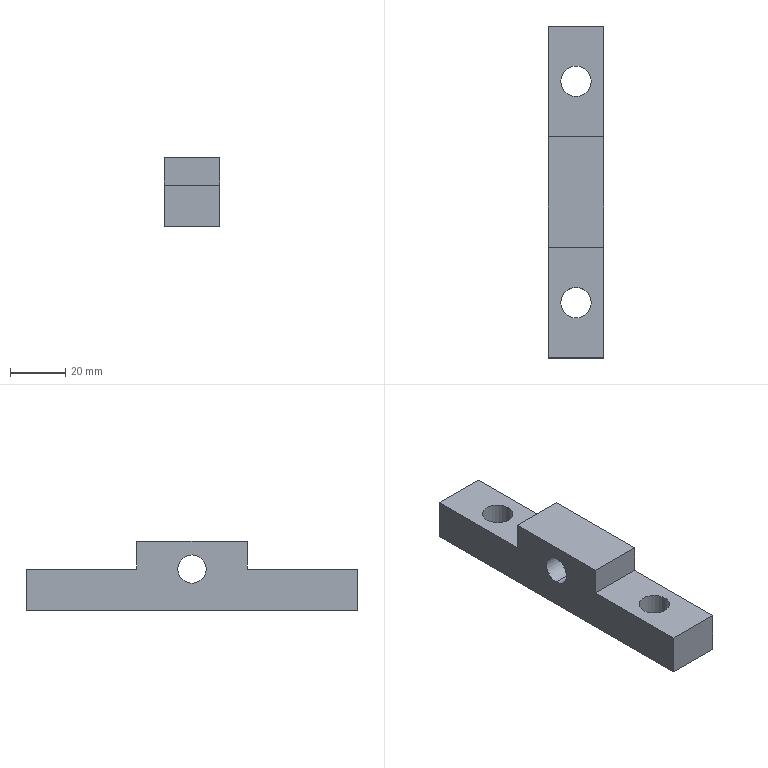Part | STEP file | Driven sprocket expansion seat | 1 solid | 16 faces | box 20 x 120 x 25 mm | volume 39515 mm3 | plane 10 | cylinder 6 | commonest cylinder face diameters 11 x4 10.2 x2
STEP:
#1=CARTESIAN_POINT('',(0.,0.,0.));
#2=DIRECTION('',(0.,0.,1.));
#3=DIRECTION('',(1.,0.,0.));
#4=AXIS2_PLACEMENT_3D('',#1,#2,#3);
#5=CARTESIAN_POINT('',(-10.,0.,9.9));
#6=VERTEX_POINT('',#5);
#7=CARTESIAN_POINT('',(10.,0.,9.9));
#8=VERTEX_POINT('',#7);
#9=CARTESIAN_POINT('',(10.,0.,9.9));
#10=DIRECTION('',(1.,0.,0.));
#11=VECTOR('',#10,1.);
#12=LINE('',#9,#11);
#13=CARTESIAN_POINT('',(10.,0.,15.));
#14=DIRECTION('',(1.,0.,0.));
#15=DIRECTION('',(0.,0.,-1.));
#16=AXIS2_PLACEMENT_3D('',#13,#14,#15);
#17=CYLINDRICAL_SURFACE('',#16,5.1);
#18=CARTESIAN_POINT('',(6.283,0.));
#19=DIRECTION('',(0.,1.));
#20=VECTOR('',#19,1.);
#21=LINE('',#18,#20);
#22=(GEOMETRIC_REPRESENTATION_CONTEXT(2)PARAMETRIC_REPRESENTATION_CONTEXT()REPRESENTATION_CONTEXT('',''));
#23=DEFINITIONAL_REPRESENTATION('',(#21),#22);
#24=PCURVE('',#17,#23);
#25=CARTESIAN_POINT('',(10.,0.,15.));
#26=DIRECTION('',(1.,0.,0.));
#27=DIRECTION('',(0.,0.,-1.));
#28=AXIS2_PLACEMENT_3D('',#25,#26,#27);
#29=CYLINDRICAL_SURFACE('',#28,5.1);
#30=CARTESIAN_POINT('',(0.,0.));
#31=DIRECTION('',(0.,1.));
#32=VECTOR('',#31,1.);
#33=LINE('',#30,#32);
#34=(GEOMETRIC_REPRESENTATION_CONTEXT(2)PARAMETRIC_REPRESENTATION_CONTEXT()REPRESENTATION_CONTEXT('',''));
#35=DEFINITIONAL_REPRESENTATION('',(#33),#34);
#36=PCURVE('',#29,#35);
#37=SURFACE_CURVE('',#12,(#24,#36),.PCURVE_S1.);
#38=EDGE_CURVE('',#6,#8,#37,.T.);
#39=ORIENTED_EDGE('',*,*,#38,.T.);
#40=CARTESIAN_POINT('',(10.,0.,20.1));
#41=VERTEX_POINT('',#40);
#42=CARTESIAN_POINT('',(10.,0.,15.));
#43=DIRECTION('',(1.,0.,0.));
#44=DIRECTION('',(0.,0.,-1.));
#45=AXIS2_PLACEMENT_3D('',#42,#43,#44);
#46=CIRCLE('',#45,5.1);
#47=CARTESIAN_POINT('',(0.,0.));
#48=DIRECTION('',(1.,0.));
#49=VECTOR('',#48,1.);
#50=LINE('',#47,#49);
#51=(GEOMETRIC_REPRESENTATION_CONTEXT(2)PARAMETRIC_REPRESENTATION_CONTEXT()REPRESENTATION_CONTEXT('',''));
#52=DEFINITIONAL_REPRESENTATION('',(#50),#51);
#53=PCURVE('',#17,#52);
#54=CARTESIAN_POINT('',(10.,60.,25.));
#55=DIRECTION('',(-1.,0.,0.));
#56=DIRECTION('',(0.,-1.,0.));
#57=AXIS2_PLACEMENT_3D('',#54,#55,#56);
#58=PLANE('',#57);
#59=CARTESIAN_POINT('',(60.,-15.1));
#60=CARTESIAN_POINT('',(51.167,-15.1));
#61=CARTESIAN_POINT('',(55.583,-7.45));
#62=CARTESIAN_POINT('',(60.,0.2));
#63=CARTESIAN_POINT('',(64.417,-7.45));
#64=CARTESIAN_POINT('',(68.833,-15.1));
#65=CARTESIAN_POINT('',(60.,-15.1));
#66=(BOUNDED_CURVE()B_SPLINE_CURVE(2,(#59,#60,#61,#62,#63,#64,#65),.UNSPECIFIED.,.T.,.F.)B_SPLINE_CURVE_WITH_KNOTS((1,2,2,2,2,1),(-2.094,0.,2.094,4.189,6.283,8.378),.UNSPECIFIED.)CURVE()GEOMETRIC_REPRESENTATION_ITEM()RATIONAL_B_SPLINE_CURVE((1.,0.5,1.,0.5,1.,0.5,1.))REPRESENTATION_ITEM(''));
#67=(GEOMETRIC_REPRESENTATION_CONTEXT(2)PARAMETRIC_REPRESENTATION_CONTEXT()REPRESENTATION_CONTEXT('',''));
#68=DEFINITIONAL_REPRESENTATION('',(#66),#67);
#69=PCURVE('',#58,#68);
#70=SURFACE_CURVE('',#46,(#53,#69),.PCURVE_S1.);
#71=EDGE_CURVE('',#41,#8,#70,.T.);
#72=ORIENTED_EDGE('',*,*,#71,.F.);
#73=CARTESIAN_POINT('',(-10.,0.,20.1));
#74=VERTEX_POINT('',#73);
#75=CARTESIAN_POINT('',(10.,0.,20.1));
#76=DIRECTION('',(1.,0.,0.));
#77=VECTOR('',#76,1.);
#78=LINE('',#75,#77);
#79=CARTESIAN_POINT('',(3.142,0.));
#80=DIRECTION('',(0.,1.));
#81=VECTOR('',#80,1.);
#82=LINE('',#79,#81);
#83=(GEOMETRIC_REPRESENTATION_CONTEXT(2)PARAMETRIC_REPRESENTATION_CONTEXT()REPRESENTATION_CONTEXT('',''));
#84=DEFINITIONAL_REPRESENTATION('',(#82),#83);
#85=PCURVE('',#17,#84);
#86=CARTESIAN_POINT('',(3.142,0.));
#87=DIRECTION('',(0.,1.));
#88=VECTOR('',#87,1.);
#89=LINE('',#86,#88);
#90=(GEOMETRIC_REPRESENTATION_CONTEXT(2)PARAMETRIC_REPRESENTATION_CONTEXT()REPRESENTATION_CONTEXT('',''));
#91=DEFINITIONAL_REPRESENTATION('',(#89),#90);
#92=PCURVE('',#29,#91);
#93=SURFACE_CURVE('',#78,(#85,#92),.PCURVE_S1.);
#94=EDGE_CURVE('',#74,#41,#93,.T.);
#95=ORIENTED_EDGE('',*,*,#94,.F.);
#96=CARTESIAN_POINT('',(-10.,0.,15.));
#97=DIRECTION('',(1.,0.,0.));
#98=DIRECTION('',(0.,0.,-1.));
#99=AXIS2_PLACEMENT_3D('',#96,#97,#98);
#100=CIRCLE('',#99,5.1);
#101=CARTESIAN_POINT('',(0.,-20.));
#102=DIRECTION('',(1.,0.));
#103=VECTOR('',#102,1.);
#104=LINE('',#101,#103);
#105=(GEOMETRIC_REPRESENTATION_CONTEXT(2)PARAMETRIC_REPRESENTATION_CONTEXT()REPRESENTATION_CONTEXT('',''));
#106=DEFINITIONAL_REPRESENTATION('',(#104),#105);
#107=PCURVE('',#17,#106);
#108=CARTESIAN_POINT('',(-10.,60.,25.));
#109=DIRECTION('',(1.,0.,0.));
#110=DIRECTION('',(0.,1.,0.));
#111=AXIS2_PLACEMENT_3D('',#108,#109,#110);
#112=PLANE('',#111);
#113=CARTESIAN_POINT('',(-60.,-10.));
#114=DIRECTION('',(0.,-1.));
#115=AXIS2_PLACEMENT_2D('',#113,#114);
#116=CIRCLE('',#115,5.1);
#117=(GEOMETRIC_REPRESENTATION_CONTEXT(2)PARAMETRIC_REPRESENTATION_CONTEXT()REPRESENTATION_CONTEXT('',''));
#118=DEFINITIONAL_REPRESENTATION('',(#116),#117);
#119=PCURVE('',#112,#118);
#120=SURFACE_CURVE('',#100,(#107,#119),.PCURVE_S1.);
#121=EDGE_CURVE('',#74,#6,#120,.T.);
#122=ORIENTED_EDGE('',*,*,#121,.T.);
#123=EDGE_LOOP('',(#39,#72,#95,#122));
#124=FACE_BOUND('',#123,.F.);
#125=ADVANCED_FACE('',(#124),#17,.F.);
#126=CARTESIAN_POINT('',(5.5,40.,0.));
#127=VERTEX_POINT('',#126);
#128=CARTESIAN_POINT('',(5.5,40.,15.));
#129=VERTEX_POINT('',#128);
#130=CARTESIAN_POINT('',(5.5,40.,25.));
#131=DIRECTION('',(0.,0.,1.));
#132=VECTOR('',#131,1.);
#133=LINE('',#130,#132);
#134=CARTESIAN_POINT('',(0.,40.,25.));
#135=DIRECTION('',(0.,0.,1.));
#136=DIRECTION('',(1.,0.,0.));
#137=AXIS2_PLACEMENT_3D('',#134,#135,#136);
#138=CYLINDRICAL_SURFACE('',#137,5.5);
#139=CARTESIAN_POINT('',(6.283,0.));
#140=DIRECTION('',(0.,1.));
#141=VECTOR('',#140,1.);
#142=LINE('',#139,#141);
#143=(GEOMETRIC_REPRESENTATION_CONTEXT(2)PARAMETRIC_REPRESENTATION_CONTEXT()REPRESENTATION_CONTEXT('',''));
#144=DEFINITIONAL_REPRESENTATION('',(#142),#143);
#145=PCURVE('',#138,#144);
#146=CARTESIAN_POINT('',(0.,40.,25.));
#147=DIRECTION('',(0.,0.,1.));
#148=DIRECTION('',(1.,0.,0.));
#149=AXIS2_PLACEMENT_3D('',#146,#147,#148);
#150=CYLINDRICAL_SURFACE('',#149,5.5);
#151=CARTESIAN_POINT('',(0.,0.));
#152=DIRECTION('',(0.,1.));
#153=VECTOR('',#152,1.);
#154=LINE('',#151,#153);
#155=(GEOMETRIC_REPRESENTATION_CONTEXT(2)PARAMETRIC_REPRESENTATION_CONTEXT()REPRESENTATION_CONTEXT('',''));
#156=DEFINITIONAL_REPRESENTATION('',(#154),#155);
#157=PCURVE('',#150,#156);
#158=SURFACE_CURVE('',#133,(#145,#157),.PCURVE_S1.);
#159=EDGE_CURVE('',#127,#129,#158,.T.);
#160=ORIENTED_EDGE('',*,*,#159,.T.);
#161=CARTESIAN_POINT('',(-5.5,40.,15.));
#162=VERTEX_POINT('',#161);
#163=CARTESIAN_POINT('',(0.,40.,15.));
#164=DIRECTION('',(0.,0.,-1.));
#165=DIRECTION('',(0.,1.,0.));
#166=AXIS2_PLACEMENT_3D('',#163,#164,#165);
#167=CIRCLE('',#166,5.5);
#168=CARTESIAN_POINT('',(7.854,-10.));
#169=DIRECTION('',(-1.,0.));
#170=VECTOR('',#169,1.);
#171=LINE('',#168,#170);
#172=(GEOMETRIC_REPRESENTATION_CONTEXT(2)PARAMETRIC_REPRESENTATION_CONTEXT()REPRESENTATION_CONTEXT('',''));
#173=DEFINITIONAL_REPRESENTATION('',(#171),#172);
#174=PCURVE('',#138,#173);
#175=CARTESIAN_POINT('',(-10.,60.,15.));
#176=DIRECTION('',(0.,0.,-1.));
#177=DIRECTION('',(0.,1.,0.));
#178=AXIS2_PLACEMENT_3D('',#175,#176,#177);
#179=PLANE('',#178);
#180=CARTESIAN_POINT('',(-20.,10.));
#181=DIRECTION('',(1.,0.));
#182=AXIS2_PLACEMENT_2D('',#180,#181);
#183=CIRCLE('',#182,5.5);
#184=(GEOMETRIC_REPRESENTATION_CONTEXT(2)PARAMETRIC_REPRESENTATION_CONTEXT()REPRESENTATION_CONTEXT('',''));
#185=DEFINITIONAL_REPRESENTATION('',(#183),#184);
#186=PCURVE('',#179,#185);
#187=SURFACE_CURVE('',#167,(#174,#186),.PCURVE_S1.);
#188=EDGE_CURVE('',#129,#162,#187,.T.);
#189=ORIENTED_EDGE('',*,*,#188,.T.);
#190=CARTESIAN_POINT('',(-5.5,40.,0.));
#191=VERTEX_POINT('',#190);
#192=CARTESIAN_POINT('',(-5.5,40.,25.));
#193=DIRECTION('',(0.,0.,1.));
#194=VECTOR('',#193,1.);
#195=LINE('',#192,#194);
#196=CARTESIAN_POINT('',(3.142,0.));
#197=DIRECTION('',(0.,1.));
#198=VECTOR('',#197,1.);
#199=LINE('',#196,#198);
#200=(GEOMETRIC_REPRESENTATION_CONTEXT(2)PARAMETRIC_REPRESENTATION_CONTEXT()REPRESENTATION_CONTEXT('',''));
#201=DEFINITIONAL_REPRESENTATION('',(#199),#200);
#202=PCURVE('',#138,#201);
#203=CARTESIAN_POINT('',(3.142,0.));
#204=DIRECTION('',(0.,1.));
#205=VECTOR('',#204,1.);
#206=LINE('',#203,#205);
#207=(GEOMETRIC_REPRESENTATION_CONTEXT(2)PARAMETRIC_REPRESENTATION_CONTEXT()REPRESENTATION_CONTEXT('',''));
#208=DEFINITIONAL_REPRESENTATION('',(#206),#207);
#209=PCURVE('',#150,#208);
#210=SURFACE_CURVE('',#195,(#202,#209),.PCURVE_S1.);
#211=EDGE_CURVE('',#191,#162,#210,.T.);
#212=ORIENTED_EDGE('',*,*,#211,.F.);
#213=CARTESIAN_POINT('',(0.,40.,0.));
#214=DIRECTION('',(0.,0.,1.));
#215=DIRECTION('',(1.,0.,0.));
#216=AXIS2_PLACEMENT_3D('',#213,#214,#215);
#217=CIRCLE('',#216,5.5);
#218=CARTESIAN_POINT('',(0.,-25.));
#219=DIRECTION('',(1.,0.));
#220=VECTOR('',#219,1.);
#221=LINE('',#218,#220);
#222=(GEOMETRIC_REPRESENTATION_CONTEXT(2)PARAMETRIC_REPRESENTATION_CONTEXT()REPRESENTATION_CONTEXT('',''));
#223=DEFINITIONAL_REPRESENTATION('',(#221),#222);
#224=PCURVE('',#138,#223);
#225=CARTESIAN_POINT('',(0.,0.,0.));
#226=DIRECTION('',(0.,0.,1.));
#227=DIRECTION('',(1.,0.,0.));
#228=AXIS2_PLACEMENT_3D('',#225,#226,#227);
#229=PLANE('',#228);
#230=CARTESIAN_POINT('',(0.,40.));
#231=DIRECTION('',(1.,0.));
#232=AXIS2_PLACEMENT_2D('',#230,#231);
#233=CIRCLE('',#232,5.5);
#234=(GEOMETRIC_REPRESENTATION_CONTEXT(2)PARAMETRIC_REPRESENTATION_CONTEXT()REPRESENTATION_CONTEXT('',''));
#235=DEFINITIONAL_REPRESENTATION('',(#233),#234);
#236=PCURVE('',#229,#235);
#237=SURFACE_CURVE('',#217,(#224,#236),.PCURVE_S1.);
#238=EDGE_CURVE('',#191,#127,#237,.T.);
#239=ORIENTED_EDGE('',*,*,#238,.T.);
#240=EDGE_LOOP('',(#160,#189,#212,#239));
#241=FACE_BOUND('',#240,.F.);
#242=ADVANCED_FACE('',(#241),#138,.F.);
#243=CARTESIAN_POINT('',(5.5,-40.,0.));
#244=VERTEX_POINT('',#243);
#245=CARTESIAN_POINT('',(5.5,-40.,15.));
#246=VERTEX_POINT('',#245);
#247=CARTESIAN_POINT('',(5.5,-40.,25.));
#248=DIRECTION('',(0.,0.,1.));
#249=VECTOR('',#248,1.);
#250=LINE('',#247,#249);
#251=CARTESIAN_POINT('',(0.,-40.,25.));
#252=DIRECTION('',(0.,0.,1.));
#253=DIRECTION('',(1.,0.,0.));
#254=AXIS2_PLACEMENT_3D('',#251,#252,#253);
#255=CYLINDRICAL_SURFACE('',#254,5.5);
#256=CARTESIAN_POINT('',(6.283,0.));
#257=DIRECTION('',(0.,1.));
#258=VECTOR('',#257,1.);
#259=LINE('',#256,#258);
#260=(GEOMETRIC_REPRESENTATION_CONTEXT(2)PARAMETRIC_REPRESENTATION_CONTEXT()REPRESENTATION_CONTEXT('',''));
#261=DEFINITIONAL_REPRESENTATION('',(#259),#260);
#262=PCURVE('',#255,#261);
#263=CARTESIAN_POINT('',(0.,-40.,25.));
#264=DIRECTION('',(0.,0.,1.));
#265=DIRECTION('',(1.,0.,0.));
#266=AXIS2_PLACEMENT_3D('',#263,#264,#265);
#267=CYLINDRICAL_SURFACE('',#266,5.5);
#268=CARTESIAN_POINT('',(0.,0.));
#269=DIRECTION('',(0.,1.));
#270=VECTOR('',#269,1.);
#271=LINE('',#268,#270);
#272=(GEOMETRIC_REPRESENTATION_CONTEXT(2)PARAMETRIC_REPRESENTATION_CONTEXT()REPRESENTATION_CONTEXT('',''));
#273=DEFINITIONAL_REPRESENTATION('',(#271),#272);
#274=PCURVE('',#267,#273);
#275=SURFACE_CURVE('',#250,(#262,#274),.PCURVE_S1.);
#276=EDGE_CURVE('',#244,#246,#275,.T.);
#277=ORIENTED_EDGE('',*,*,#276,.T.);
#278=CARTESIAN_POINT('',(-5.5,-40.,15.));
#279=VERTEX_POINT('',#278);
#280=CARTESIAN_POINT('',(0.,-40.,15.));
#281=DIRECTION('',(0.,0.,-1.));
#282=DIRECTION('',(0.,1.,0.));
#283=AXIS2_PLACEMENT_3D('',#280,#281,#282);
#284=CIRCLE('',#283,5.5);
#285=CARTESIAN_POINT('',(7.854,-10.));
#286=DIRECTION('',(-1.,0.));
#287=VECTOR('',#286,1.);
#288=LINE('',#285,#287);
#289=(GEOMETRIC_REPRESENTATION_CONTEXT(2)PARAMETRIC_REPRESENTATION_CONTEXT()REPRESENTATION_CONTEXT('',''));
#290=DEFINITIONAL_REPRESENTATION('',(#288),#289);
#291=PCURVE('',#255,#290);
#292=CARTESIAN_POINT('',(-10.,-60.,15.));
#293=DIRECTION('',(0.,0.,-1.));
#294=DIRECTION('',(0.,1.,0.));
#295=AXIS2_PLACEMENT_3D('',#292,#293,#294);
#296=PLANE('',#295);
#297=CARTESIAN_POINT('',(20.,10.));
#298=DIRECTION('',(1.,0.));
#299=AXIS2_PLACEMENT_2D('',#297,#298);
#300=CIRCLE('',#299,5.5);
#301=(GEOMETRIC_REPRESENTATION_CONTEXT(2)PARAMETRIC_REPRESENTATION_CONTEXT()REPRESENTATION_CONTEXT('',''));
#302=DEFINITIONAL_REPRESENTATION('',(#300),#301);
#303=PCURVE('',#296,#302);
#304=SURFACE_CURVE('',#284,(#291,#303),.PCURVE_S1.);
#305=EDGE_CURVE('',#246,#279,#304,.T.);
#306=ORIENTED_EDGE('',*,*,#305,.T.);
#307=CARTESIAN_POINT('',(-5.5,-40.,0.));
#308=VERTEX_POINT('',#307);
#309=CARTESIAN_POINT('',(-5.5,-40.,25.));
#310=DIRECTION('',(0.,0.,1.));
#311=VECTOR('',#310,1.);
#312=LINE('',#309,#311);
#313=CARTESIAN_POINT('',(3.142,0.));
#314=DIRECTION('',(0.,1.));
#315=VECTOR('',#314,1.);
#316=LINE('',#313,#315);
#317=(GEOMETRIC_REPRESENTATION_CONTEXT(2)PARAMETRIC_REPRESENTATION_CONTEXT()REPRESENTATION_CONTEXT('',''));
#318=DEFINITIONAL_REPRESENTATION('',(#316),#317);
#319=PCURVE('',#255,#318);
#320=CARTESIAN_POINT('',(3.142,0.));
#321=DIRECTION('',(0.,1.));
#322=VECTOR('',#321,1.);
#323=LINE('',#320,#322);
#324=(GEOMETRIC_REPRESENTATION_CONTEXT(2)PARAMETRIC_REPRESENTATION_CONTEXT()REPRESENTATION_CONTEXT('',''));
#325=DEFINITIONAL_REPRESENTATION('',(#323),#324);
#326=PCURVE('',#267,#325);
#327=SURFACE_CURVE('',#312,(#319,#326),.PCURVE_S1.);
#328=EDGE_CURVE('',#308,#279,#327,.T.);
#329=ORIENTED_EDGE('',*,*,#328,.F.);
#330=CARTESIAN_POINT('',(0.,-40.,0.));
#331=DIRECTION('',(0.,0.,1.));
#332=DIRECTION('',(1.,0.,0.));
#333=AXIS2_PLACEMENT_3D('',#330,#331,#332);
#334=CIRCLE('',#333,5.5);
#335=CARTESIAN_POINT('',(0.,-25.));
#336=DIRECTION('',(1.,0.));
#337=VECTOR('',#336,1.);
#338=LINE('',#335,#337);
#339=(GEOMETRIC_REPRESENTATION_CONTEXT(2)PARAMETRIC_REPRESENTATION_CONTEXT()REPRESENTATION_CONTEXT('',''));
#340=DEFINITIONAL_REPRESENTATION('',(#338),#339);
#341=PCURVE('',#255,#340);
#342=CARTESIAN_POINT('',(0.,-40.));
#343=DIRECTION('',(1.,0.));
#344=AXIS2_PLACEMENT_2D('',#342,#343);
#345=CIRCLE('',#344,5.5);
#346=(GEOMETRIC_REPRESENTATION_CONTEXT(2)PARAMETRIC_REPRESENTATION_CONTEXT()REPRESENTATION_CONTEXT('',''));
#347=DEFINITIONAL_REPRESENTATION('',(#345),#346);
#348=PCURVE('',#229,#347);
#349=SURFACE_CURVE('',#334,(#341,#348),.PCURVE_S1.);
#350=EDGE_CURVE('',#308,#244,#349,.T.);
#351=ORIENTED_EDGE('',*,*,#350,.T.);
#352=EDGE_LOOP('',(#277,#306,#329,#351));
#353=FACE_BOUND('',#352,.F.);
#354=ADVANCED_FACE('',(#353),#255,.F.);
#355=CARTESIAN_POINT('',(10.,0.,15.));
#356=DIRECTION('',(1.,0.,0.));
#357=DIRECTION('',(0.,0.,-1.));
#358=AXIS2_PLACEMENT_3D('',#355,#356,#357);
#359=CIRCLE('',#358,5.1);
#360=CARTESIAN_POINT('',(60.,-15.1));
#361=CARTESIAN_POINT('',(51.167,-15.1));
#362=CARTESIAN_POINT('',(55.583,-7.45));
#363=CARTESIAN_POINT('',(60.,0.2));
#364=CARTESIAN_POINT('',(64.417,-7.45));
#365=CARTESIAN_POINT('',(68.833,-15.1));
#366=CARTESIAN_POINT('',(60.,-15.1));
#367=(BOUNDED_CURVE()B_SPLINE_CURVE(2,(#360,#361,#362,#363,#364,#365,#366),.UNSPECIFIED.,.T.,.F.)B_SPLINE_CURVE_WITH_KNOTS((1,2,2,2,2,1),(-2.094,0.,2.094,4.189,6.283,8.378),.UNSPECIFIED.)CURVE()GEOMETRIC_REPRESENTATION_ITEM()RATIONAL_B_SPLINE_CURVE((1.,0.5,1.,0.5,1.,0.5,1.))REPRESENTATION_ITEM(''));
#368=(GEOMETRIC_REPRESENTATION_CONTEXT(2)PARAMETRIC_REPRESENTATION_CONTEXT()REPRESENTATION_CONTEXT('',''));
#369=DEFINITIONAL_REPRESENTATION('',(#367),#368);
#370=PCURVE('',#58,#369);
#371=CARTESIAN_POINT('',(0.,0.));
#372=DIRECTION('',(1.,0.));
#373=VECTOR('',#372,1.);
#374=LINE('',#371,#373);
#375=(GEOMETRIC_REPRESENTATION_CONTEXT(2)PARAMETRIC_REPRESENTATION_CONTEXT()REPRESENTATION_CONTEXT('',''));
#376=DEFINITIONAL_REPRESENTATION('',(#374),#375);
#377=PCURVE('',#29,#376);
#378=SURFACE_CURVE('',#359,(#370,#377),.PCURVE_S1.);
#379=EDGE_CURVE('',#8,#41,#378,.T.);
#380=ORIENTED_EDGE('',*,*,#379,.F.);
#381=ORIENTED_EDGE('',*,*,#71,.F.);
#382=EDGE_LOOP('',(#380,#381));
#383=FACE_BOUND('',#382,.T.);
#384=CARTESIAN_POINT('',(10.,-20.,25.));
#385=VERTEX_POINT('',#384);
#386=CARTESIAN_POINT('',(10.,20.,25.));
#387=VERTEX_POINT('',#386);
#388=CARTESIAN_POINT('',(10.,60.,25.));
#389=DIRECTION('',(0.,1.,0.));
#390=VECTOR('',#389,1.);
#391=LINE('',#388,#390);
#392=CARTESIAN_POINT('',(0.,0.));
#393=DIRECTION('',(-1.,0.));
#394=VECTOR('',#393,1.);
#395=LINE('',#392,#394);
#396=(GEOMETRIC_REPRESENTATION_CONTEXT(2)PARAMETRIC_REPRESENTATION_CONTEXT()REPRESENTATION_CONTEXT('',''));
#397=DEFINITIONAL_REPRESENTATION('',(#395),#396);
#398=PCURVE('',#58,#397);
#399=CARTESIAN_POINT('',(0.,0.,25.));
#400=DIRECTION('',(0.,0.,1.));
#401=DIRECTION('',(1.,0.,0.));
#402=AXIS2_PLACEMENT_3D('',#399,#400,#401);
#403=PLANE('',#402);
#404=CARTESIAN_POINT('',(10.,60.));
#405=DIRECTION('',(0.,1.));
#406=VECTOR('',#405,1.);
#407=LINE('',#404,#406);
#408=(GEOMETRIC_REPRESENTATION_CONTEXT(2)PARAMETRIC_REPRESENTATION_CONTEXT()REPRESENTATION_CONTEXT('',''));
#409=DEFINITIONAL_REPRESENTATION('',(#407),#408);
#410=PCURVE('',#403,#409);
#411=SURFACE_CURVE('',#391,(#398,#410),.PCURVE_S1.);
#412=EDGE_CURVE('',#385,#387,#411,.T.);
#413=ORIENTED_EDGE('',*,*,#412,.F.);
#414=CARTESIAN_POINT('',(10.,-20.,15.));
#415=VERTEX_POINT('',#414);
#416=CARTESIAN_POINT('',(10.,-20.,25.));
#417=DIRECTION('',(0.,0.,1.));
#418=VECTOR('',#417,1.);
#419=LINE('',#416,#418);
#420=CARTESIAN_POINT('',(80.,0.));
#421=DIRECTION('',(0.,1.));
#422=VECTOR('',#421,1.);
#423=LINE('',#420,#422);
#424=(GEOMETRIC_REPRESENTATION_CONTEXT(2)PARAMETRIC_REPRESENTATION_CONTEXT()REPRESENTATION_CONTEXT('',''));
#425=DEFINITIONAL_REPRESENTATION('',(#423),#424);
#426=PCURVE('',#58,#425);
#427=CARTESIAN_POINT('',(-10.,-20.,25.));
#428=DIRECTION('',(0.,1.,0.));
#429=DIRECTION('',(-1.,0.,0.));
#430=AXIS2_PLACEMENT_3D('',#427,#428,#429);
#431=PLANE('',#430);
#432=CARTESIAN_POINT('',(-20.,0.));
#433=DIRECTION('',(0.,1.));
#434=VECTOR('',#433,1.);
#435=LINE('',#432,#434);
#436=(GEOMETRIC_REPRESENTATION_CONTEXT(2)PARAMETRIC_REPRESENTATION_CONTEXT()REPRESENTATION_CONTEXT('',''));
#437=DEFINITIONAL_REPRESENTATION('',(#435),#436);
#438=PCURVE('',#431,#437);
#439=SURFACE_CURVE('',#419,(#426,#438),.PCURVE_S1.);
#440=EDGE_CURVE('',#415,#385,#439,.T.);
#441=ORIENTED_EDGE('',*,*,#440,.F.);
#442=CARTESIAN_POINT('',(10.,-60.,15.));
#443=VERTEX_POINT('',#442);
#444=CARTESIAN_POINT('',(10.,-60.,15.));
#445=DIRECTION('',(0.,1.,0.));
#446=VECTOR('',#445,1.);
#447=LINE('',#444,#446);
#448=CARTESIAN_POINT('',(120.,-10.));
#449=DIRECTION('',(-1.,0.));
#450=VECTOR('',#449,1.);
#451=LINE('',#448,#450);
#452=(GEOMETRIC_REPRESENTATION_CONTEXT(2)PARAMETRIC_REPRESENTATION_CONTEXT()REPRESENTATION_CONTEXT('',''));
#453=DEFINITIONAL_REPRESENTATION('',(#451),#452);
#454=PCURVE('',#58,#453);
#455=CARTESIAN_POINT('',(0.,20.));
#456=DIRECTION('',(1.,0.));
#457=VECTOR('',#456,1.);
#458=LINE('',#455,#457);
#459=(GEOMETRIC_REPRESENTATION_CONTEXT(2)PARAMETRIC_REPRESENTATION_CONTEXT()REPRESENTATION_CONTEXT('',''));
#460=DEFINITIONAL_REPRESENTATION('',(#458),#459);
#461=PCURVE('',#296,#460);
#462=SURFACE_CURVE('',#447,(#454,#461),.PCURVE_S1.);
#463=EDGE_CURVE('',#443,#415,#462,.T.);
#464=ORIENTED_EDGE('',*,*,#463,.F.);
#465=CARTESIAN_POINT('',(10.,-60.,0.));
#466=VERTEX_POINT('',#465);
#467=CARTESIAN_POINT('',(10.,-60.,25.));
#468=DIRECTION('',(0.,0.,-1.));
#469=VECTOR('',#468,1.);
#470=LINE('',#467,#469);
#471=CARTESIAN_POINT('',(120.,0.));
#472=DIRECTION('',(0.,-1.));
#473=VECTOR('',#472,1.);
#474=LINE('',#471,#473);
#475=(GEOMETRIC_REPRESENTATION_CONTEXT(2)PARAMETRIC_REPRESENTATION_CONTEXT()REPRESENTATION_CONTEXT('',''));
#476=DEFINITIONAL_REPRESENTATION('',(#474),#475);
#477=PCURVE('',#58,#476);
#478=CARTESIAN_POINT('',(-10.,-60.,25.));
#479=DIRECTION('',(0.,1.,0.));
#480=DIRECTION('',(0.,0.,1.));
#481=AXIS2_PLACEMENT_3D('',#478,#479,#480);
#482=PLANE('',#481);
#483=CARTESIAN_POINT('',(0.,20.));
#484=DIRECTION('',(-1.,0.));
#485=VECTOR('',#484,1.);
#486=LINE('',#483,#485);
#487=(GEOMETRIC_REPRESENTATION_CONTEXT(2)PARAMETRIC_REPRESENTATION_CONTEXT()REPRESENTATION_CONTEXT('',''));
#488=DEFINITIONAL_REPRESENTATION('',(#486),#487);
#489=PCURVE('',#482,#488);
#490=SURFACE_CURVE('',#470,(#477,#489),.PCURVE_S1.);
#491=EDGE_CURVE('',#443,#466,#490,.T.);
#492=ORIENTED_EDGE('',*,*,#491,.T.);
#493=CARTESIAN_POINT('',(10.,60.,0.));
#494=VERTEX_POINT('',#493);
#495=CARTESIAN_POINT('',(10.,60.,0.));
#496=DIRECTION('',(0.,1.,0.));
#497=VECTOR('',#496,1.);
#498=LINE('',#495,#497);
#499=CARTESIAN_POINT('',(0.,-25.));
#500=DIRECTION('',(-1.,0.));
#501=VECTOR('',#500,1.);
#502=LINE('',#499,#501);
#503=(GEOMETRIC_REPRESENTATION_CONTEXT(2)PARAMETRIC_REPRESENTATION_CONTEXT()REPRESENTATION_CONTEXT('',''));
#504=DEFINITIONAL_REPRESENTATION('',(#502),#503);
#505=PCURVE('',#58,#504);
#506=CARTESIAN_POINT('',(10.,60.));
#507=DIRECTION('',(0.,1.));
#508=VECTOR('',#507,1.);
#509=LINE('',#506,#508);
#510=(GEOMETRIC_REPRESENTATION_CONTEXT(2)PARAMETRIC_REPRESENTATION_CONTEXT()REPRESENTATION_CONTEXT('',''));
#511=DEFINITIONAL_REPRESENTATION('',(#509),#510);
#512=PCURVE('',#229,#511);
#513=SURFACE_CURVE('',#498,(#505,#512),.PCURVE_S1.);
#514=EDGE_CURVE('',#466,#494,#513,.T.);
#515=ORIENTED_EDGE('',*,*,#514,.T.);
#516=CARTESIAN_POINT('',(10.,60.,15.));
#517=VERTEX_POINT('',#516);
#518=CARTESIAN_POINT('',(10.,60.,25.));
#519=DIRECTION('',(0.,0.,-1.));
#520=VECTOR('',#519,1.);
#521=LINE('',#518,#520);
#522=CARTESIAN_POINT('',(0.,0.));
#523=DIRECTION('',(0.,-1.));
#524=VECTOR('',#523,1.);
#525=LINE('',#522,#524);
#526=(GEOMETRIC_REPRESENTATION_CONTEXT(2)PARAMETRIC_REPRESENTATION_CONTEXT()REPRESENTATION_CONTEXT('',''));
#527=DEFINITIONAL_REPRESENTATION('',(#525),#526);
#528=PCURVE('',#58,#527);
#529=CARTESIAN_POINT('',(-10.,60.,25.));
#530=DIRECTION('',(0.,-1.,0.));
#531=DIRECTION('',(0.,0.,-1.));
#532=AXIS2_PLACEMENT_3D('',#529,#530,#531);
#533=PLANE('',#532);
#534=CARTESIAN_POINT('',(0.,20.));
#535=DIRECTION('',(1.,0.));
#536=VECTOR('',#535,1.);
#537=LINE('',#534,#536);
#538=(GEOMETRIC_REPRESENTATION_CONTEXT(2)PARAMETRIC_REPRESENTATION_CONTEXT()REPRESENTATION_CONTEXT('',''));
#539=DEFINITIONAL_REPRESENTATION('',(#537),#538);
#540=PCURVE('',#533,#539);
#541=SURFACE_CURVE('',#521,(#528,#540),.PCURVE_S1.);
#542=EDGE_CURVE('',#517,#494,#541,.T.);
#543=ORIENTED_EDGE('',*,*,#542,.F.);
#544=CARTESIAN_POINT('',(10.,20.,15.));
#545=VERTEX_POINT('',#544);
#546=CARTESIAN_POINT('',(10.,60.,15.));
#547=DIRECTION('',(0.,1.,0.));
#548=VECTOR('',#547,1.);
#549=LINE('',#546,#548);
#550=CARTESIAN_POINT('',(0.,-10.));
#551=DIRECTION('',(-1.,0.));
#552=VECTOR('',#551,1.);
#553=LINE('',#550,#552);
#554=(GEOMETRIC_REPRESENTATION_CONTEXT(2)PARAMETRIC_REPRESENTATION_CONTEXT()REPRESENTATION_CONTEXT('',''));
#555=DEFINITIONAL_REPRESENTATION('',(#553),#554);
#556=PCURVE('',#58,#555);
#557=CARTESIAN_POINT('',(0.,20.));
#558=DIRECTION('',(1.,0.));
#559=VECTOR('',#558,1.);
#560=LINE('',#557,#559);
#561=(GEOMETRIC_REPRESENTATION_CONTEXT(2)PARAMETRIC_REPRESENTATION_CONTEXT()REPRESENTATION_CONTEXT('',''));
#562=DEFINITIONAL_REPRESENTATION('',(#560),#561);
#563=PCURVE('',#179,#562);
#564=SURFACE_CURVE('',#549,(#556,#563),.PCURVE_S1.);
#565=EDGE_CURVE('',#545,#517,#564,.T.);
#566=ORIENTED_EDGE('',*,*,#565,.F.);
#567=CARTESIAN_POINT('',(10.,20.,25.));
#568=DIRECTION('',(0.,0.,-1.));
#569=VECTOR('',#568,1.);
#570=LINE('',#567,#569);
#571=CARTESIAN_POINT('',(40.,0.));
#572=DIRECTION('',(0.,-1.));
#573=VECTOR('',#572,1.);
#574=LINE('',#571,#573);
#575=(GEOMETRIC_REPRESENTATION_CONTEXT(2)PARAMETRIC_REPRESENTATION_CONTEXT()REPRESENTATION_CONTEXT('',''));
#576=DEFINITIONAL_REPRESENTATION('',(#574),#575);
#577=PCURVE('',#58,#576);
#578=CARTESIAN_POINT('',(-10.,20.,25.));
#579=DIRECTION('',(0.,-1.,0.));
#580=DIRECTION('',(1.,0.,0.));
#581=AXIS2_PLACEMENT_3D('',#578,#579,#580);
#582=PLANE('',#581);
#583=CARTESIAN_POINT('',(20.,0.));
#584=DIRECTION('',(0.,-1.));
#585=VECTOR('',#584,1.);
#586=LINE('',#583,#585);
#587=(GEOMETRIC_REPRESENTATION_CONTEXT(2)PARAMETRIC_REPRESENTATION_CONTEXT()REPRESENTATION_CONTEXT('',''));
#588=DEFINITIONAL_REPRESENTATION('',(#586),#587);
#589=PCURVE('',#582,#588);
#590=SURFACE_CURVE('',#570,(#577,#589),.PCURVE_S1.);
#591=EDGE_CURVE('',#387,#545,#590,.T.);
#592=ORIENTED_EDGE('',*,*,#591,.F.);
#593=EDGE_LOOP('',(#413,#441,#464,#492,#515,#543,#566,#592));
#594=FACE_BOUND('',#593,.T.);
#595=ADVANCED_FACE('',(#383,#594),#58,.F.);
#596=CARTESIAN_POINT('',(-10.,60.,15.));
#597=VERTEX_POINT('',#596);
#598=CARTESIAN_POINT('',(-10.,60.,0.));
#599=VERTEX_POINT('',#598);
#600=CARTESIAN_POINT('',(-10.,60.,25.));
#601=DIRECTION('',(0.,0.,-1.));
#602=VECTOR('',#601,1.);
#603=LINE('',#600,#602);
#604=CARTESIAN_POINT('',(0.,0.));
#605=DIRECTION('',(1.,0.));
#606=VECTOR('',#605,1.);
#607=LINE('',#604,#606);
#608=(GEOMETRIC_REPRESENTATION_CONTEXT(2)PARAMETRIC_REPRESENTATION_CONTEXT()REPRESENTATION_CONTEXT('',''));
#609=DEFINITIONAL_REPRESENTATION('',(#607),#608);
#610=PCURVE('',#533,#609);
#611=CARTESIAN_POINT('',(0.,0.));
#612=DIRECTION('',(0.,-1.));
#613=VECTOR('',#612,1.);
#614=LINE('',#611,#613);
#615=(GEOMETRIC_REPRESENTATION_CONTEXT(2)PARAMETRIC_REPRESENTATION_CONTEXT()REPRESENTATION_CONTEXT('',''));
#616=DEFINITIONAL_REPRESENTATION('',(#614),#615);
#617=PCURVE('',#112,#616);
#618=SURFACE_CURVE('',#603,(#610,#617),.PCURVE_S1.);
#619=EDGE_CURVE('',#597,#599,#618,.T.);
#620=ORIENTED_EDGE('',*,*,#619,.F.);
#621=CARTESIAN_POINT('',(-10.,60.,15.));
#622=DIRECTION('',(1.,0.,0.));
#623=VECTOR('',#622,1.);
#624=LINE('',#621,#623);
#625=CARTESIAN_POINT('',(10.,0.));
#626=DIRECTION('',(0.,1.));
#627=VECTOR('',#626,1.);
#628=LINE('',#625,#627);
#629=(GEOMETRIC_REPRESENTATION_CONTEXT(2)PARAMETRIC_REPRESENTATION_CONTEXT()REPRESENTATION_CONTEXT('',''));
#630=DEFINITIONAL_REPRESENTATION('',(#628),#629);
#631=PCURVE('',#533,#630);
#632=CARTESIAN_POINT('',(0.,0.));
#633=DIRECTION('',(0.,1.));
#634=VECTOR('',#633,1.);
#635=LINE('',#632,#634);
#636=(GEOMETRIC_REPRESENTATION_CONTEXT(2)PARAMETRIC_REPRESENTATION_CONTEXT()REPRESENTATION_CONTEXT('',''));
#637=DEFINITIONAL_REPRESENTATION('',(#635),#636);
#638=PCURVE('',#179,#637);
#639=SURFACE_CURVE('',#624,(#631,#638),.PCURVE_S1.);
#640=EDGE_CURVE('',#597,#517,#639,.T.);
#641=ORIENTED_EDGE('',*,*,#640,.T.);
#642=ORIENTED_EDGE('',*,*,#542,.T.);
#643=CARTESIAN_POINT('',(-10.,60.,0.));
#644=DIRECTION('',(-1.,0.,0.));
#645=VECTOR('',#644,1.);
#646=LINE('',#643,#645);
#647=CARTESIAN_POINT('',(25.,0.));
#648=DIRECTION('',(0.,-1.));
#649=VECTOR('',#648,1.);
#650=LINE('',#647,#649);
#651=(GEOMETRIC_REPRESENTATION_CONTEXT(2)PARAMETRIC_REPRESENTATION_CONTEXT()REPRESENTATION_CONTEXT('',''));
#652=DEFINITIONAL_REPRESENTATION('',(#650),#651);
#653=PCURVE('',#533,#652);
#654=CARTESIAN_POINT('',(-10.,60.));
#655=DIRECTION('',(-1.,0.));
#656=VECTOR('',#655,1.);
#657=LINE('',#654,#656);
#658=(GEOMETRIC_REPRESENTATION_CONTEXT(2)PARAMETRIC_REPRESENTATION_CONTEXT()REPRESENTATION_CONTEXT('',''));
#659=DEFINITIONAL_REPRESENTATION('',(#657),#658);
#660=PCURVE('',#229,#659);
#661=SURFACE_CURVE('',#646,(#653,#660),.PCURVE_S1.);
#662=EDGE_CURVE('',#494,#599,#661,.T.);
#663=ORIENTED_EDGE('',*,*,#662,.T.);
#664=EDGE_LOOP('',(#620,#641,#642,#663));
#665=FACE_BOUND('',#664,.T.);
#666=ADVANCED_FACE('',(#665),#533,.F.);
#667=CARTESIAN_POINT('',(-10.,0.,15.));
#668=DIRECTION('',(1.,0.,0.));
#669=DIRECTION('',(0.,0.,-1.));
#670=AXIS2_PLACEMENT_3D('',#667,#668,#669);
#671=CIRCLE('',#670,5.1);
#672=CARTESIAN_POINT('',(-60.,-10.));
#673=DIRECTION('',(0.,-1.));
#674=AXIS2_PLACEMENT_2D('',#672,#673);
#675=CIRCLE('',#674,5.1);
#676=(GEOMETRIC_REPRESENTATION_CONTEXT(2)PARAMETRIC_REPRESENTATION_CONTEXT()REPRESENTATION_CONTEXT('',''));
#677=DEFINITIONAL_REPRESENTATION('',(#675),#676);
#678=PCURVE('',#112,#677);
#679=CARTESIAN_POINT('',(0.,-20.));
#680=DIRECTION('',(1.,0.));
#681=VECTOR('',#680,1.);
#682=LINE('',#679,#681);
#683=(GEOMETRIC_REPRESENTATION_CONTEXT(2)PARAMETRIC_REPRESENTATION_CONTEXT()REPRESENTATION_CONTEXT('',''));
#684=DEFINITIONAL_REPRESENTATION('',(#682),#683);
#685=PCURVE('',#29,#684);
#686=SURFACE_CURVE('',#671,(#678,#685),.PCURVE_S1.);
#687=EDGE_CURVE('',#6,#74,#686,.T.);
#688=ORIENTED_EDGE('',*,*,#687,.T.);
#689=ORIENTED_EDGE('',*,*,#121,.T.);
#690=EDGE_LOOP('',(#688,#689));
#691=FACE_BOUND('',#690,.T.);
#692=CARTESIAN_POINT('',(-10.,-60.,15.));
#693=VERTEX_POINT('',#692);
#694=CARTESIAN_POINT('',(-10.,-20.,15.));
#695=VERTEX_POINT('',#694);
#696=CARTESIAN_POINT('',(-10.,-60.,15.));
#697=DIRECTION('',(0.,1.,0.));
#698=VECTOR('',#697,1.);
#699=LINE('',#696,#698);
#700=CARTESIAN_POINT('',(-120.,-10.));
#701=DIRECTION('',(1.,0.));
#702=VECTOR('',#701,1.);
#703=LINE('',#700,#702);
#704=(GEOMETRIC_REPRESENTATION_CONTEXT(2)PARAMETRIC_REPRESENTATION_CONTEXT()REPRESENTATION_CONTEXT('',''));
#705=DEFINITIONAL_REPRESENTATION('',(#703),#704);
#706=PCURVE('',#112,#705);
#707=CARTESIAN_POINT('',(0.,0.));
#708=DIRECTION('',(1.,0.));
#709=VECTOR('',#708,1.);
#710=LINE('',#707,#709);
#711=(GEOMETRIC_REPRESENTATION_CONTEXT(2)PARAMETRIC_REPRESENTATION_CONTEXT()REPRESENTATION_CONTEXT('',''));
#712=DEFINITIONAL_REPRESENTATION('',(#710),#711);
#713=PCURVE('',#296,#712);
#714=SURFACE_CURVE('',#699,(#706,#713),.PCURVE_S1.);
#715=EDGE_CURVE('',#693,#695,#714,.T.);
#716=ORIENTED_EDGE('',*,*,#715,.T.);
#717=CARTESIAN_POINT('',(-10.,-20.,25.));
#718=VERTEX_POINT('',#717);
#719=CARTESIAN_POINT('',(-10.,-20.,25.));
#720=DIRECTION('',(0.,0.,1.));
#721=VECTOR('',#720,1.);
#722=LINE('',#719,#721);
#723=CARTESIAN_POINT('',(-80.,0.));
#724=DIRECTION('',(0.,1.));
#725=VECTOR('',#724,1.);
#726=LINE('',#723,#725);
#727=(GEOMETRIC_REPRESENTATION_CONTEXT(2)PARAMETRIC_REPRESENTATION_CONTEXT()REPRESENTATION_CONTEXT('',''));
#728=DEFINITIONAL_REPRESENTATION('',(#726),#727);
#729=PCURVE('',#112,#728);
#730=CARTESIAN_POINT('',(0.,0.));
#731=DIRECTION('',(0.,1.));
#732=VECTOR('',#731,1.);
#733=LINE('',#730,#732);
#734=(GEOMETRIC_REPRESENTATION_CONTEXT(2)PARAMETRIC_REPRESENTATION_CONTEXT()REPRESENTATION_CONTEXT('',''));
#735=DEFINITIONAL_REPRESENTATION('',(#733),#734);
#736=PCURVE('',#431,#735);
#737=SURFACE_CURVE('',#722,(#729,#736),.PCURVE_S1.);
#738=EDGE_CURVE('',#695,#718,#737,.T.);
#739=ORIENTED_EDGE('',*,*,#738,.T.);
#740=CARTESIAN_POINT('',(-10.,20.,25.));
#741=VERTEX_POINT('',#740);
#742=CARTESIAN_POINT('',(-10.,60.,25.));
#743=DIRECTION('',(0.,-1.,0.));
#744=VECTOR('',#743,1.);
#745=LINE('',#742,#744);
#746=CARTESIAN_POINT('',(0.,0.));
#747=DIRECTION('',(-1.,0.));
#748=VECTOR('',#747,1.);
#749=LINE('',#746,#748);
#750=(GEOMETRIC_REPRESENTATION_CONTEXT(2)PARAMETRIC_REPRESENTATION_CONTEXT()REPRESENTATION_CONTEXT('',''));
#751=DEFINITIONAL_REPRESENTATION('',(#749),#750);
#752=PCURVE('',#112,#751);
#753=CARTESIAN_POINT('',(-10.,60.));
#754=DIRECTION('',(0.,-1.));
#755=VECTOR('',#754,1.);
#756=LINE('',#753,#755);
#757=(GEOMETRIC_REPRESENTATION_CONTEXT(2)PARAMETRIC_REPRESENTATION_CONTEXT()REPRESENTATION_CONTEXT('',''));
#758=DEFINITIONAL_REPRESENTATION('',(#756),#757);
#759=PCURVE('',#403,#758);
#760=SURFACE_CURVE('',#745,(#752,#759),.PCURVE_S1.);
#761=EDGE_CURVE('',#741,#718,#760,.T.);
#762=ORIENTED_EDGE('',*,*,#761,.F.);
#763=CARTESIAN_POINT('',(-10.,20.,15.));
#764=VERTEX_POINT('',#763);
#765=CARTESIAN_POINT('',(-10.,20.,25.));
#766=DIRECTION('',(0.,0.,-1.));
#767=VECTOR('',#766,1.);
#768=LINE('',#765,#767);
#769=CARTESIAN_POINT('',(-40.,0.));
#770=DIRECTION('',(0.,-1.));
#771=VECTOR('',#770,1.);
#772=LINE('',#769,#771);
#773=(GEOMETRIC_REPRESENTATION_CONTEXT(2)PARAMETRIC_REPRESENTATION_CONTEXT()REPRESENTATION_CONTEXT('',''));
#774=DEFINITIONAL_REPRESENTATION('',(#772),#773);
#775=PCURVE('',#112,#774);
#776=CARTESIAN_POINT('',(0.,0.));
#777=DIRECTION('',(0.,-1.));
#778=VECTOR('',#777,1.);
#779=LINE('',#776,#778);
#780=(GEOMETRIC_REPRESENTATION_CONTEXT(2)PARAMETRIC_REPRESENTATION_CONTEXT()REPRESENTATION_CONTEXT('',''));
#781=DEFINITIONAL_REPRESENTATION('',(#779),#780);
#782=PCURVE('',#582,#781);
#783=SURFACE_CURVE('',#768,(#775,#782),.PCURVE_S1.);
#784=EDGE_CURVE('',#741,#764,#783,.T.);
#785=ORIENTED_EDGE('',*,*,#784,.T.);
#786=CARTESIAN_POINT('',(-10.,60.,15.));
#787=DIRECTION('',(0.,1.,0.));
#788=VECTOR('',#787,1.);
#789=LINE('',#786,#788);
#790=CARTESIAN_POINT('',(0.,-10.));
#791=DIRECTION('',(1.,0.));
#792=VECTOR('',#791,1.);
#793=LINE('',#790,#792);
#794=(GEOMETRIC_REPRESENTATION_CONTEXT(2)PARAMETRIC_REPRESENTATION_CONTEXT()REPRESENTATION_CONTEXT('',''));
#795=DEFINITIONAL_REPRESENTATION('',(#793),#794);
#796=PCURVE('',#112,#795);
#797=CARTESIAN_POINT('',(0.,0.));
#798=DIRECTION('',(1.,0.));
#799=VECTOR('',#798,1.);
#800=LINE('',#797,#799);
#801=(GEOMETRIC_REPRESENTATION_CONTEXT(2)PARAMETRIC_REPRESENTATION_CONTEXT()REPRESENTATION_CONTEXT('',''));
#802=DEFINITIONAL_REPRESENTATION('',(#800),#801);
#803=PCURVE('',#179,#802);
#804=SURFACE_CURVE('',#789,(#796,#803),.PCURVE_S1.);
#805=EDGE_CURVE('',#764,#597,#804,.T.);
#806=ORIENTED_EDGE('',*,*,#805,.T.);
#807=ORIENTED_EDGE('',*,*,#619,.T.);
#808=CARTESIAN_POINT('',(-10.,-60.,0.));
#809=VERTEX_POINT('',#808);
#810=CARTESIAN_POINT('',(-10.,60.,0.));
#811=DIRECTION('',(0.,-1.,0.));
#812=VECTOR('',#811,1.);
#813=LINE('',#810,#812);
#814=CARTESIAN_POINT('',(0.,-25.));
#815=DIRECTION('',(-1.,0.));
#816=VECTOR('',#815,1.);
#817=LINE('',#814,#816);
#818=(GEOMETRIC_REPRESENTATION_CONTEXT(2)PARAMETRIC_REPRESENTATION_CONTEXT()REPRESENTATION_CONTEXT('',''));
#819=DEFINITIONAL_REPRESENTATION('',(#817),#818);
#820=PCURVE('',#112,#819);
#821=CARTESIAN_POINT('',(-10.,60.));
#822=DIRECTION('',(0.,-1.));
#823=VECTOR('',#822,1.);
#824=LINE('',#821,#823);
#825=(GEOMETRIC_REPRESENTATION_CONTEXT(2)PARAMETRIC_REPRESENTATION_CONTEXT()REPRESENTATION_CONTEXT('',''));
#826=DEFINITIONAL_REPRESENTATION('',(#824),#825);
#827=PCURVE('',#229,#826);
#828=SURFACE_CURVE('',#813,(#820,#827),.PCURVE_S1.);
#829=EDGE_CURVE('',#599,#809,#828,.T.);
#830=ORIENTED_EDGE('',*,*,#829,.T.);
#831=CARTESIAN_POINT('',(-10.,-60.,25.));
#832=DIRECTION('',(0.,0.,-1.));
#833=VECTOR('',#832,1.);
#834=LINE('',#831,#833);
#835=CARTESIAN_POINT('',(-120.,0.));
#836=DIRECTION('',(0.,-1.));
#837=VECTOR('',#836,1.);
#838=LINE('',#835,#837);
#839=(GEOMETRIC_REPRESENTATION_CONTEXT(2)PARAMETRIC_REPRESENTATION_CONTEXT()REPRESENTATION_CONTEXT('',''));
#840=DEFINITIONAL_REPRESENTATION('',(#838),#839);
#841=PCURVE('',#112,#840);
#842=CARTESIAN_POINT('',(0.,0.));
#843=DIRECTION('',(-1.,0.));
#844=VECTOR('',#843,1.);
#845=LINE('',#842,#844);
#846=(GEOMETRIC_REPRESENTATION_CONTEXT(2)PARAMETRIC_REPRESENTATION_CONTEXT()REPRESENTATION_CONTEXT('',''));
#847=DEFINITIONAL_REPRESENTATION('',(#845),#846);
#848=PCURVE('',#482,#847);
#849=SURFACE_CURVE('',#834,(#841,#848),.PCURVE_S1.);
#850=EDGE_CURVE('',#693,#809,#849,.T.);
#851=ORIENTED_EDGE('',*,*,#850,.F.);
#852=EDGE_LOOP('',(#716,#739,#762,#785,#806,#807,#830,#851));
#853=FACE_BOUND('',#852,.T.);
#854=ADVANCED_FACE('',(#691,#853),#112,.F.);
#855=ORIENTED_EDGE('',*,*,#491,.F.);
#856=CARTESIAN_POINT('',(-10.,-60.,15.));
#857=DIRECTION('',(1.,0.,0.));
#858=VECTOR('',#857,1.);
#859=LINE('',#856,#858);
#860=CARTESIAN_POINT('',(-10.,0.));
#861=DIRECTION('',(0.,1.));
#862=VECTOR('',#861,1.);
#863=LINE('',#860,#862);
#864=(GEOMETRIC_REPRESENTATION_CONTEXT(2)PARAMETRIC_REPRESENTATION_CONTEXT()REPRESENTATION_CONTEXT('',''));
#865=DEFINITIONAL_REPRESENTATION('',(#863),#864);
#866=PCURVE('',#482,#865);
#867=CARTESIAN_POINT('',(0.,0.));
#868=DIRECTION('',(0.,1.));
#869=VECTOR('',#868,1.);
#870=LINE('',#867,#869);
#871=(GEOMETRIC_REPRESENTATION_CONTEXT(2)PARAMETRIC_REPRESENTATION_CONTEXT()REPRESENTATION_CONTEXT('',''));
#872=DEFINITIONAL_REPRESENTATION('',(#870),#871);
#873=PCURVE('',#296,#872);
#874=SURFACE_CURVE('',#859,(#866,#873),.PCURVE_S1.);
#875=EDGE_CURVE('',#693,#443,#874,.T.);
#876=ORIENTED_EDGE('',*,*,#875,.F.);
#877=ORIENTED_EDGE('',*,*,#850,.T.);
#878=CARTESIAN_POINT('',(-10.,-60.,0.));
#879=DIRECTION('',(1.,0.,0.));
#880=VECTOR('',#879,1.);
#881=LINE('',#878,#880);
#882=CARTESIAN_POINT('',(-25.,0.));
#883=DIRECTION('',(0.,1.));
#884=VECTOR('',#883,1.);
#885=LINE('',#882,#884);
#886=(GEOMETRIC_REPRESENTATION_CONTEXT(2)PARAMETRIC_REPRESENTATION_CONTEXT()REPRESENTATION_CONTEXT('',''));
#887=DEFINITIONAL_REPRESENTATION('',(#885),#886);
#888=PCURVE('',#482,#887);
#889=CARTESIAN_POINT('',(-10.,-60.));
#890=DIRECTION('',(1.,0.));
#891=VECTOR('',#890,1.);
#892=LINE('',#889,#891);
#893=(GEOMETRIC_REPRESENTATION_CONTEXT(2)PARAMETRIC_REPRESENTATION_CONTEXT()REPRESENTATION_CONTEXT('',''));
#894=DEFINITIONAL_REPRESENTATION('',(#892),#893);
#895=PCURVE('',#229,#894);
#896=SURFACE_CURVE('',#881,(#888,#895),.PCURVE_S1.);
#897=EDGE_CURVE('',#809,#466,#896,.T.);
#898=ORIENTED_EDGE('',*,*,#897,.T.);
#899=EDGE_LOOP('',(#855,#876,#877,#898));
#900=FACE_BOUND('',#899,.T.);
#901=ADVANCED_FACE('',(#900),#482,.F.);
#902=CARTESIAN_POINT('',(-10.,-20.,25.));
#903=DIRECTION('',(1.,0.,0.));
#904=VECTOR('',#903,1.);
#905=LINE('',#902,#904);
#906=CARTESIAN_POINT('',(-10.,-20.));
#907=DIRECTION('',(1.,0.));
#908=VECTOR('',#907,1.);
#909=LINE('',#906,#908);
#910=(GEOMETRIC_REPRESENTATION_CONTEXT(2)PARAMETRIC_REPRESENTATION_CONTEXT()REPRESENTATION_CONTEXT('',''));
#911=DEFINITIONAL_REPRESENTATION('',(#909),#910);
#912=PCURVE('',#403,#911);
#913=CARTESIAN_POINT('',(0.,0.));
#914=DIRECTION('',(-1.,0.));
#915=VECTOR('',#914,1.);
#916=LINE('',#913,#915);
#917=(GEOMETRIC_REPRESENTATION_CONTEXT(2)PARAMETRIC_REPRESENTATION_CONTEXT()REPRESENTATION_CONTEXT('',''));
#918=DEFINITIONAL_REPRESENTATION('',(#916),#917);
#919=PCURVE('',#431,#918);
#920=SURFACE_CURVE('',#905,(#912,#919),.PCURVE_S1.);
#921=EDGE_CURVE('',#718,#385,#920,.T.);
#922=ORIENTED_EDGE('',*,*,#921,.T.);
#923=ORIENTED_EDGE('',*,*,#412,.T.);
#924=CARTESIAN_POINT('',(-10.,20.,25.));
#925=DIRECTION('',(1.,0.,0.));
#926=VECTOR('',#925,1.);
#927=LINE('',#924,#926);
#928=CARTESIAN_POINT('',(-10.,20.));
#929=DIRECTION('',(1.,0.));
#930=VECTOR('',#929,1.);
#931=LINE('',#928,#930);
#932=(GEOMETRIC_REPRESENTATION_CONTEXT(2)PARAMETRIC_REPRESENTATION_CONTEXT()REPRESENTATION_CONTEXT('',''));
#933=DEFINITIONAL_REPRESENTATION('',(#931),#932);
#934=PCURVE('',#403,#933);
#935=CARTESIAN_POINT('',(0.,0.));
#936=DIRECTION('',(1.,0.));
#937=VECTOR('',#936,1.);
#938=LINE('',#935,#937);
#939=(GEOMETRIC_REPRESENTATION_CONTEXT(2)PARAMETRIC_REPRESENTATION_CONTEXT()REPRESENTATION_CONTEXT('',''));
#940=DEFINITIONAL_REPRESENTATION('',(#938),#939);
#941=PCURVE('',#582,#940);
#942=SURFACE_CURVE('',#927,(#934,#941),.PCURVE_S1.);
#943=EDGE_CURVE('',#741,#387,#942,.T.);
#944=ORIENTED_EDGE('',*,*,#943,.F.);
#945=ORIENTED_EDGE('',*,*,#761,.T.);
#946=EDGE_LOOP('',(#922,#923,#944,#945));
#947=FACE_BOUND('',#946,.T.);
#948=ADVANCED_FACE('',(#947),#403,.T.);
#949=CARTESIAN_POINT('',(0.,40.,0.));
#950=DIRECTION('',(0.,0.,1.));
#951=DIRECTION('',(1.,0.,0.));
#952=AXIS2_PLACEMENT_3D('',#949,#950,#951);
#953=CIRCLE('',#952,5.5);
#954=CARTESIAN_POINT('',(0.,40.));
#955=DIRECTION('',(1.,0.));
#956=AXIS2_PLACEMENT_2D('',#954,#955);
#957=CIRCLE('',#956,5.5);
#958=(GEOMETRIC_REPRESENTATION_CONTEXT(2)PARAMETRIC_REPRESENTATION_CONTEXT()REPRESENTATION_CONTEXT('',''));
#959=DEFINITIONAL_REPRESENTATION('',(#957),#958);
#960=PCURVE('',#229,#959);
#961=CARTESIAN_POINT('',(0.,-25.));
#962=DIRECTION('',(1.,0.));
#963=VECTOR('',#962,1.);
#964=LINE('',#961,#963);
#965=(GEOMETRIC_REPRESENTATION_CONTEXT(2)PARAMETRIC_REPRESENTATION_CONTEXT()REPRESENTATION_CONTEXT('',''));
#966=DEFINITIONAL_REPRESENTATION('',(#964),#965);
#967=PCURVE('',#150,#966);
#968=SURFACE_CURVE('',#953,(#960,#967),.PCURVE_S1.);
#969=EDGE_CURVE('',#127,#191,#968,.T.);
#970=ORIENTED_EDGE('',*,*,#969,.T.);
#971=ORIENTED_EDGE('',*,*,#238,.T.);
#972=EDGE_LOOP('',(#970,#971));
#973=FACE_BOUND('',#972,.T.);
#974=CARTESIAN_POINT('',(0.,-40.,0.));
#975=DIRECTION('',(0.,0.,1.));
#976=DIRECTION('',(1.,0.,0.));
#977=AXIS2_PLACEMENT_3D('',#974,#975,#976);
#978=CIRCLE('',#977,5.5);
#979=CARTESIAN_POINT('',(0.,-40.));
#980=DIRECTION('',(1.,0.));
#981=AXIS2_PLACEMENT_2D('',#979,#980);
#982=CIRCLE('',#981,5.5);
#983=(GEOMETRIC_REPRESENTATION_CONTEXT(2)PARAMETRIC_REPRESENTATION_CONTEXT()REPRESENTATION_CONTEXT('',''));
#984=DEFINITIONAL_REPRESENTATION('',(#982),#983);
#985=PCURVE('',#229,#984);
#986=CARTESIAN_POINT('',(0.,-25.));
#987=DIRECTION('',(1.,0.));
#988=VECTOR('',#987,1.);
#989=LINE('',#986,#988);
#990=(GEOMETRIC_REPRESENTATION_CONTEXT(2)PARAMETRIC_REPRESENTATION_CONTEXT()REPRESENTATION_CONTEXT('',''));
#991=DEFINITIONAL_REPRESENTATION('',(#989),#990);
#992=PCURVE('',#267,#991);
#993=SURFACE_CURVE('',#978,(#985,#992),.PCURVE_S1.);
#994=EDGE_CURVE('',#244,#308,#993,.T.);
#995=ORIENTED_EDGE('',*,*,#994,.T.);
#996=ORIENTED_EDGE('',*,*,#350,.T.);
#997=EDGE_LOOP('',(#995,#996));
#998=FACE_BOUND('',#997,.T.);
#999=ORIENTED_EDGE('',*,*,#514,.F.);
#1000=ORIENTED_EDGE('',*,*,#897,.F.);
#1001=ORIENTED_EDGE('',*,*,#829,.F.);
#1002=ORIENTED_EDGE('',*,*,#662,.F.);
#1003=EDGE_LOOP('',(#999,#1000,#1001,#1002));
#1004=FACE_BOUND('',#1003,.T.);
#1005=ADVANCED_FACE('',(#973,#998,#1004),#229,.F.);
#1006=ORIENTED_EDGE('',*,*,#188,.T.);
#1007=CARTESIAN_POINT('',(0.,40.,15.));
#1008=DIRECTION('',(0.,0.,-1.));
#1009=DIRECTION('',(0.,1.,0.));
#1010=AXIS2_PLACEMENT_3D('',#1007,#1008,#1009);
#1011=CIRCLE('',#1010,5.5);
#1012=CARTESIAN_POINT('',(-20.,10.));
#1013=DIRECTION('',(1.,0.));
#1014=AXIS2_PLACEMENT_2D('',#1012,#1013);
#1015=CIRCLE('',#1014,5.5);
#1016=(GEOMETRIC_REPRESENTATION_CONTEXT(2)PARAMETRIC_REPRESENTATION_CONTEXT()REPRESENTATION_CONTEXT('',''));
#1017=DEFINITIONAL_REPRESENTATION('',(#1015),#1016);
#1018=PCURVE('',#179,#1017);
#1019=CARTESIAN_POINT('',(7.854,-10.));
#1020=DIRECTION('',(-1.,0.));
#1021=VECTOR('',#1020,1.);
#1022=LINE('',#1019,#1021);
#1023=(GEOMETRIC_REPRESENTATION_CONTEXT(2)PARAMETRIC_REPRESENTATION_CONTEXT()REPRESENTATION_CONTEXT('',''));
#1024=DEFINITIONAL_REPRESENTATION('',(#1022),#1023);
#1025=PCURVE('',#150,#1024);
#1026=SURFACE_CURVE('',#1011,(#1018,#1025),.PCURVE_S1.);
#1027=EDGE_CURVE('',#162,#129,#1026,.T.);
#1028=ORIENTED_EDGE('',*,*,#1027,.T.);
#1029=EDGE_LOOP('',(#1006,#1028));
#1030=FACE_BOUND('',#1029,.T.);
#1031=ORIENTED_EDGE('',*,*,#565,.T.);
#1032=ORIENTED_EDGE('',*,*,#640,.F.);
#1033=ORIENTED_EDGE('',*,*,#805,.F.);
#1034=CARTESIAN_POINT('',(-10.,20.,15.));
#1035=DIRECTION('',(1.,0.,0.));
#1036=VECTOR('',#1035,1.);
#1037=LINE('',#1034,#1036);
#1038=CARTESIAN_POINT('',(-40.,0.));
#1039=DIRECTION('',(0.,1.));
#1040=VECTOR('',#1039,1.);
#1041=LINE('',#1038,#1040);
#1042=(GEOMETRIC_REPRESENTATION_CONTEXT(2)PARAMETRIC_REPRESENTATION_CONTEXT()REPRESENTATION_CONTEXT('',''));
#1043=DEFINITIONAL_REPRESENTATION('',(#1041),#1042);
#1044=PCURVE('',#179,#1043);
#1045=CARTESIAN_POINT('',(0.,-10.));
#1046=DIRECTION('',(1.,0.));
#1047=VECTOR('',#1046,1.);
#1048=LINE('',#1045,#1047);
#1049=(GEOMETRIC_REPRESENTATION_CONTEXT(2)PARAMETRIC_REPRESENTATION_CONTEXT()REPRESENTATION_CONTEXT('',''));
#1050=DEFINITIONAL_REPRESENTATION('',(#1048),#1049);
#1051=PCURVE('',#582,#1050);
#1052=SURFACE_CURVE('',#1037,(#1044,#1051),.PCURVE_S1.);
#1053=EDGE_CURVE('',#764,#545,#1052,.T.);
#1054=ORIENTED_EDGE('',*,*,#1053,.T.);
#1055=EDGE_LOOP('',(#1031,#1032,#1033,#1054));
#1056=FACE_BOUND('',#1055,.T.);
#1057=ADVANCED_FACE('',(#1030,#1056),#179,.F.);
#1058=ORIENTED_EDGE('',*,*,#591,.T.);
#1059=ORIENTED_EDGE('',*,*,#1053,.F.);
#1060=ORIENTED_EDGE('',*,*,#784,.F.);
#1061=ORIENTED_EDGE('',*,*,#943,.T.);
#1062=EDGE_LOOP('',(#1058,#1059,#1060,#1061));
#1063=FACE_BOUND('',#1062,.T.);
#1064=ADVANCED_FACE('',(#1063),#582,.F.);
#1065=ORIENTED_EDGE('',*,*,#440,.T.);
#1066=ORIENTED_EDGE('',*,*,#921,.F.);
#1067=ORIENTED_EDGE('',*,*,#738,.F.);
#1068=CARTESIAN_POINT('',(-10.,-20.,15.));
#1069=DIRECTION('',(1.,0.,0.));
#1070=VECTOR('',#1069,1.);
#1071=LINE('',#1068,#1070);
#1072=CARTESIAN_POINT('',(0.,-10.));
#1073=DIRECTION('',(-1.,0.));
#1074=VECTOR('',#1073,1.);
#1075=LINE('',#1072,#1074);
#1076=(GEOMETRIC_REPRESENTATION_CONTEXT(2)PARAMETRIC_REPRESENTATION_CONTEXT()REPRESENTATION_CONTEXT('',''));
#1077=DEFINITIONAL_REPRESENTATION('',(#1075),#1076);
#1078=PCURVE('',#431,#1077);
#1079=CARTESIAN_POINT('',(40.,0.));
#1080=DIRECTION('',(0.,1.));
#1081=VECTOR('',#1080,1.);
#1082=LINE('',#1079,#1081);
#1083=(GEOMETRIC_REPRESENTATION_CONTEXT(2)PARAMETRIC_REPRESENTATION_CONTEXT()REPRESENTATION_CONTEXT('',''));
#1084=DEFINITIONAL_REPRESENTATION('',(#1082),#1083);
#1085=PCURVE('',#296,#1084);
#1086=SURFACE_CURVE('',#1071,(#1078,#1085),.PCURVE_S1.);
#1087=EDGE_CURVE('',#695,#415,#1086,.T.);
#1088=ORIENTED_EDGE('',*,*,#1087,.T.);
#1089=EDGE_LOOP('',(#1065,#1066,#1067,#1088));
#1090=FACE_BOUND('',#1089,.T.);
#1091=ADVANCED_FACE('',(#1090),#431,.F.);
#1092=ORIENTED_EDGE('',*,*,#305,.T.);
#1093=CARTESIAN_POINT('',(0.,-40.,15.));
#1094=DIRECTION('',(0.,0.,-1.));
#1095=DIRECTION('',(0.,1.,0.));
#1096=AXIS2_PLACEMENT_3D('',#1093,#1094,#1095);
#1097=CIRCLE('',#1096,5.5);
#1098=CARTESIAN_POINT('',(20.,10.));
#1099=DIRECTION('',(1.,0.));
#1100=AXIS2_PLACEMENT_2D('',#1098,#1099);
#1101=CIRCLE('',#1100,5.5);
#1102=(GEOMETRIC_REPRESENTATION_CONTEXT(2)PARAMETRIC_REPRESENTATION_CONTEXT()REPRESENTATION_CONTEXT('',''));
#1103=DEFINITIONAL_REPRESENTATION('',(#1101),#1102);
#1104=PCURVE('',#296,#1103);
#1105=CARTESIAN_POINT('',(7.854,-10.));
#1106=DIRECTION('',(-1.,0.));
#1107=VECTOR('',#1106,1.);
#1108=LINE('',#1105,#1107);
#1109=(GEOMETRIC_REPRESENTATION_CONTEXT(2)PARAMETRIC_REPRESENTATION_CONTEXT()REPRESENTATION_CONTEXT('',''));
#1110=DEFINITIONAL_REPRESENTATION('',(#1108),#1109);
#1111=PCURVE('',#267,#1110);
#1112=SURFACE_CURVE('',#1097,(#1104,#1111),.PCURVE_S1.);
#1113=EDGE_CURVE('',#279,#246,#1112,.T.);
#1114=ORIENTED_EDGE('',*,*,#1113,.T.);
#1115=EDGE_LOOP('',(#1092,#1114));
#1116=FACE_BOUND('',#1115,.T.);
#1117=ORIENTED_EDGE('',*,*,#463,.T.);
#1118=ORIENTED_EDGE('',*,*,#1087,.F.);
#1119=ORIENTED_EDGE('',*,*,#715,.F.);
#1120=ORIENTED_EDGE('',*,*,#875,.T.);
#1121=EDGE_LOOP('',(#1117,#1118,#1119,#1120));
#1122=FACE_BOUND('',#1121,.T.);
#1123=ADVANCED_FACE('',(#1116,#1122),#296,.F.);
#1124=ORIENTED_EDGE('',*,*,#1113,.T.);
#1125=ORIENTED_EDGE('',*,*,#276,.F.);
#1126=ORIENTED_EDGE('',*,*,#994,.T.);
#1127=ORIENTED_EDGE('',*,*,#328,.T.);
#1128=EDGE_LOOP('',(#1124,#1125,#1126,#1127));
#1129=FACE_BOUND('',#1128,.F.);
#1130=ADVANCED_FACE('',(#1129),#267,.F.);
#1131=ORIENTED_EDGE('',*,*,#1027,.T.);
#1132=ORIENTED_EDGE('',*,*,#159,.F.);
#1133=ORIENTED_EDGE('',*,*,#969,.T.);
#1134=ORIENTED_EDGE('',*,*,#211,.T.);
#1135=EDGE_LOOP('',(#1131,#1132,#1133,#1134));
#1136=FACE_BOUND('',#1135,.F.);
#1137=ADVANCED_FACE('',(#1136),#150,.F.);
#1138=ORIENTED_EDGE('',*,*,#379,.F.);
#1139=ORIENTED_EDGE('',*,*,#38,.F.);
#1140=ORIENTED_EDGE('',*,*,#687,.T.);
#1141=ORIENTED_EDGE('',*,*,#94,.T.);
#1142=EDGE_LOOP('',(#1138,#1139,#1140,#1141));
#1143=FACE_BOUND('',#1142,.F.);
#1144=ADVANCED_FACE('',(#1143),#29,.F.);
#1145=CLOSED_SHELL('',(#125,#242,#354,#595,#666,#854,#901,#948,#1005,#1057,#1064,#1091,#1123,#1130,#1137,#1144));
#1146=MANIFOLD_SOLID_BREP('',#1145);
#1147=(LENGTH_UNIT()NAMED_UNIT(*)SI_UNIT(.MILLI.,.METRE.));
#1148=UNCERTAINTY_MEASURE_WITH_UNIT(LENGTH_MEASURE(0.0000001),#1147,'','');
#1149=(NAMED_UNIT(*)PLANE_ANGLE_UNIT()SI_UNIT($,.RADIAN.));
#1150=(NAMED_UNIT(*)SI_UNIT($,.STERADIAN.)SOLID_ANGLE_UNIT());
#1151=(GEOMETRIC_REPRESENTATION_CONTEXT(3)GLOBAL_UNCERTAINTY_ASSIGNED_CONTEXT((#1148))GLOBAL_UNIT_ASSIGNED_CONTEXT((#1147,#1149,#1150))REPRESENTATION_CONTEXT('',''));
#1152=ADVANCED_BREP_SHAPE_REPRESENTATION('',(#4,#1146),#1151);